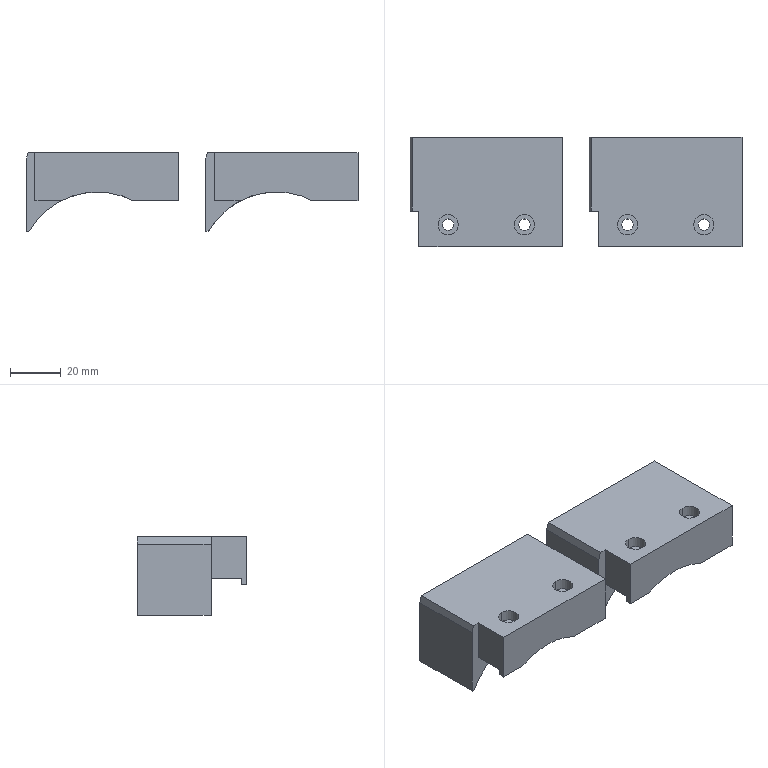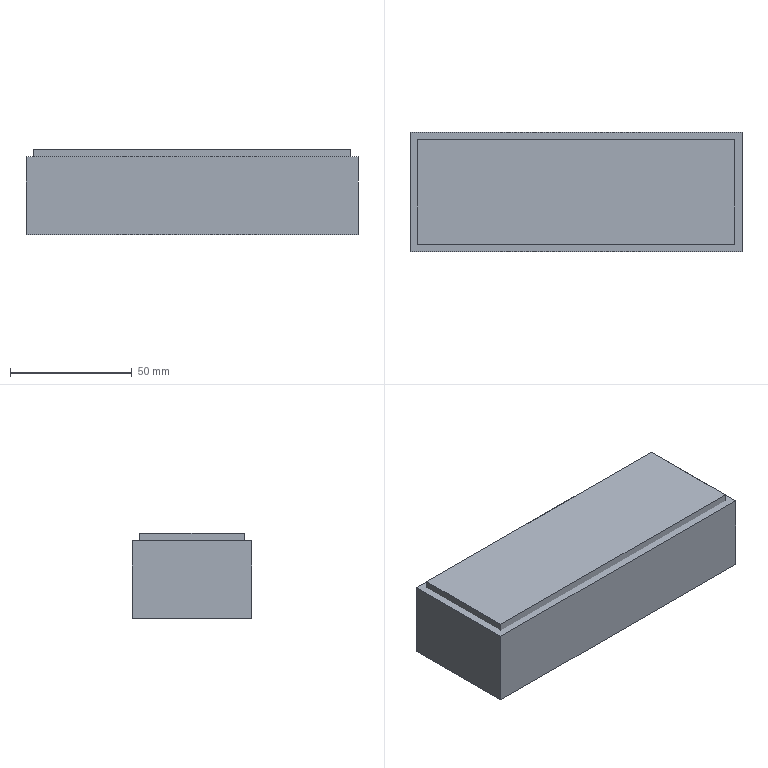CAM job | NX | 3-axis milling, drilling | part box 130.5 x 43 x 31 mm | stock box 136.5 x 49 x 35 mm
Operations:
program,operation,operation_type,tool,method,geometry_group,spindle_rpm,surface_speed,feed_per_tooth,feed_cut,feed_plunge,cut_length_mm,path_length_mm,cut_time_min,machine_time_min
1-135-50-35毛胚-虎钳,FLOOR_WALL,VolumeBased25DMillingOperation,D63,METHOD,A,6500.0,1286.0,0.0962,1250.0,100.0,211.5,265.5,0.1692,0.1746
1-135-50-35毛胚-虎钳,DRILLING_COPY_1,Operation,D6A45,METHOD,A,3000.0,56.0,0.0333,200.0,0.0,20.4,210.71,0.102,0.121
1-135-50-35毛胚-虎钳,DRILLING_COPY_1_COPY_COPY_COPY_COPY,Operation,4.5ZT,METHOD,A,2000.0,20.0,0.0375,150.0,0.0,85.408,340.726,0.5694,0.5949
1-135-50-35毛胚-虎钳,HOLE_MILLING,CylinderMilling,D6,METHOD,A,7000.0,131.0,0.1071,1500.0,100.0,284.779,640.879,0.1899,0.2255
1-135-50-35毛胚-虎钳,ZLEVEL_PROFILE,ZLevelMilling,D10,METHOD,A,7000.0,219.0,0.2143,3000.0,1000.0,14850.816,15167.844,5.014,5.046
1-135-50-35毛胚-虎钳,ZLEVEL_PROFILE_COPY_1_COPY_COPY_COPY_COPY_2_COPY,ZLevelMilling,D6A45,METHOD,A,7000.0,131.0,0.0714,1000.0,1000.0,495.74,1162.339,0.4957,0.5624
1-135-50-35毛胚-虎钳,ZLEVEL_PROFILE_COPY_COPY_1,ZLevelMilling,D10JING,METHOD,A,7000.0,219.0,0.0714,1000.0,100.0,962.437,1271.012,0.9624,0.9933
2-135-50-35毛胚-虎钳,FLOOR_WALL_COPY,VolumeBased25DMillingOperation,D63,METHOD,B,6500.0,1286.0,0.0962,1250.0,100.0,822.0,1624.501,0.6576,0.7379
2-135-50-35毛胚-虎钳,CAVITY_MILL,CavityMilling,D10,METHOD,B,7000.0,439.0,0.1571,2200.0,1000.0,13825.543,14116.774,6.723,6.76
2-135-50-35毛胚-虎钳,FLOOR_WALL_1_COPY_1,VolumeBased25DMillingOperation,D10JING,METHOD,B,7000.0,87.0,0.0714,1000.0,100.0,1243.43,2252.387,1.243,1.344
2-135-50-35毛胚-虎钳,FIXED_CONTOUR,SurfaceContour,R2,METHOD,B,7000.0,87.0,0.2143,3000.0,1000.0,30498.297,30702.274,10.171,10.192
2-135-50-35毛胚-虎钳,ZLEVEL_PROFILE_COPY_1_COPY_COPY_COPY_COPY_2_COPY_COPY,ZLevelMilling,D6A45,METHOD,B,7000.0,131.0,0.0714,1000.0,1000.0,279.649,1003.305,0.2796,0.352
2-135-50-35毛胚-虎钳,ZLEVEL_PROFILE_COPY_1_COPY_COPY_COPY_COPY_2_COPY_COPY_COPY,ZLevelMilling,D6A45,METHOD,B,7000.0,131.0,0.0714,1000.0,1000.0,60.88,1235.061,0.0609,0.1783